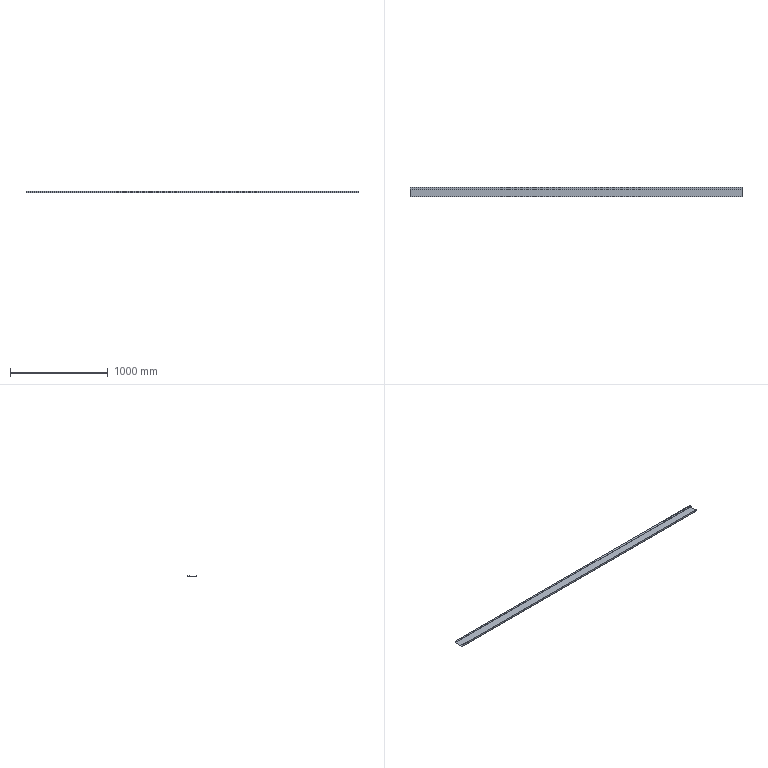Part | STEP file | Powder bin toe plate 7 | 1 solid | 18 faces | box 3390 x 100 x 20 mm | volume 779259 mm3 | plane 12 | cylinder 6 | commonest cylinder face diameters 2 x3 5 x3
STEP:
#1=CARTESIAN_POINT('',(0.,0.,0.));
#2=DIRECTION('',(0.,0.,1.));
#3=DIRECTION('',(1.,0.,0.));
#4=AXIS2_PLACEMENT_3D('',#1,#2,#3);
#5=CARTESIAN_POINT('',(-1695.,1.5,2.5));
#6=VERTEX_POINT('',#5);
#7=CARTESIAN_POINT('',(-1695.,1.5,20.));
#8=VERTEX_POINT('',#7);
#9=CARTESIAN_POINT('',(-1695.,1.5,2.5));
#10=DIRECTION('',(0.,0.,1.));
#11=VECTOR('',#10,1.);
#12=LINE('',#9,#11);
#13=CARTESIAN_POINT('',(1695.,1.5,2.5));
#14=DIRECTION('',(0.,-1.,0.));
#15=DIRECTION('',(0.,0.,-1.));
#16=AXIS2_PLACEMENT_3D('',#13,#14,#15);
#17=PLANE('',#16);
#18=CARTESIAN_POINT('',(0.,-3390.));
#19=DIRECTION('',(-1.,0.));
#20=VECTOR('',#19,1.);
#21=LINE('',#18,#20);
#22=(GEOMETRIC_REPRESENTATION_CONTEXT(2)PARAMETRIC_REPRESENTATION_CONTEXT()REPRESENTATION_CONTEXT('',''));
#23=DEFINITIONAL_REPRESENTATION('',(#21),#22);
#24=PCURVE('',#17,#23);
#25=CARTESIAN_POINT('',(-1695.,2.5,2.5));
#26=DIRECTION('',(-1.,0.,0.));
#27=DIRECTION('',(0.,0.,1.));
#28=AXIS2_PLACEMENT_3D('',#25,#26,#27);
#29=PLANE('',#28);
#30=CARTESIAN_POINT('',(0.,-1.));
#31=DIRECTION('',(1.,0.));
#32=VECTOR('',#31,1.);
#33=LINE('',#30,#32);
#34=(GEOMETRIC_REPRESENTATION_CONTEXT(2)PARAMETRIC_REPRESENTATION_CONTEXT()REPRESENTATION_CONTEXT('',''));
#35=DEFINITIONAL_REPRESENTATION('',(#33),#34);
#36=PCURVE('',#29,#35);
#37=SURFACE_CURVE('',#12,(#24,#36),.PCURVE_S1.);
#38=EDGE_CURVE('',#6,#8,#37,.T.);
#39=ORIENTED_EDGE('',*,*,#38,.T.);
#40=CARTESIAN_POINT('',(1695.,1.5,20.));
#41=VERTEX_POINT('',#40);
#42=CARTESIAN_POINT('',(1695.,1.5,20.));
#43=DIRECTION('',(-1.,0.,0.));
#44=VECTOR('',#43,1.);
#45=LINE('',#42,#44);
#46=CARTESIAN_POINT('',(-17.5,0.));
#47=DIRECTION('',(0.,-1.));
#48=VECTOR('',#47,1.);
#49=LINE('',#46,#48);
#50=(GEOMETRIC_REPRESENTATION_CONTEXT(2)PARAMETRIC_REPRESENTATION_CONTEXT()REPRESENTATION_CONTEXT('',''));
#51=DEFINITIONAL_REPRESENTATION('',(#49),#50);
#52=PCURVE('',#17,#51);
#53=CARTESIAN_POINT('',(1695.,0.,20.));
#54=DIRECTION('',(0.,0.,1.));
#55=DIRECTION('',(1.,0.,0.));
#56=AXIS2_PLACEMENT_3D('',#53,#54,#55);
#57=PLANE('',#56);
#58=CARTESIAN_POINT('',(0.,1.5));
#59=DIRECTION('',(-1.,0.));
#60=VECTOR('',#59,1.);
#61=LINE('',#58,#60);
#62=(GEOMETRIC_REPRESENTATION_CONTEXT(2)PARAMETRIC_REPRESENTATION_CONTEXT()REPRESENTATION_CONTEXT('',''));
#63=DEFINITIONAL_REPRESENTATION('',(#61),#62);
#64=PCURVE('',#57,#63);
#65=SURFACE_CURVE('',#45,(#52,#64),.PCURVE_S1.);
#66=EDGE_CURVE('',#41,#8,#65,.T.);
#67=ORIENTED_EDGE('',*,*,#66,.F.);
#68=CARTESIAN_POINT('',(1695.,1.5,2.5));
#69=VERTEX_POINT('',#68);
#70=CARTESIAN_POINT('',(1695.,1.5,2.5));
#71=DIRECTION('',(0.,0.,1.));
#72=VECTOR('',#71,1.);
#73=LINE('',#70,#72);
#74=CARTESIAN_POINT('',(0.,0.));
#75=DIRECTION('',(-1.,0.));
#76=VECTOR('',#75,1.);
#77=LINE('',#74,#76);
#78=(GEOMETRIC_REPRESENTATION_CONTEXT(2)PARAMETRIC_REPRESENTATION_CONTEXT()REPRESENTATION_CONTEXT('',''));
#79=DEFINITIONAL_REPRESENTATION('',(#77),#78);
#80=PCURVE('',#17,#79);
#81=CARTESIAN_POINT('',(1695.,2.5,2.5));
#82=DIRECTION('',(-1.,0.,0.));
#83=DIRECTION('',(0.,0.,1.));
#84=AXIS2_PLACEMENT_3D('',#81,#82,#83);
#85=PLANE('',#84);
#86=CARTESIAN_POINT('',(0.,-1.));
#87=DIRECTION('',(1.,0.));
#88=VECTOR('',#87,1.);
#89=LINE('',#86,#88);
#90=(GEOMETRIC_REPRESENTATION_CONTEXT(2)PARAMETRIC_REPRESENTATION_CONTEXT()REPRESENTATION_CONTEXT('',''));
#91=DEFINITIONAL_REPRESENTATION('',(#89),#90);
#92=PCURVE('',#85,#91);
#93=SURFACE_CURVE('',#73,(#80,#92),.PCURVE_S1.);
#94=EDGE_CURVE('',#69,#41,#93,.T.);
#95=ORIENTED_EDGE('',*,*,#94,.F.);
#96=CARTESIAN_POINT('',(1695.,1.5,2.5));
#97=DIRECTION('',(-1.,0.,0.));
#98=VECTOR('',#97,1.);
#99=LINE('',#96,#98);
#100=CARTESIAN_POINT('',(0.,0.));
#101=DIRECTION('',(0.,-1.));
#102=VECTOR('',#101,1.);
#103=LINE('',#100,#102);
#104=(GEOMETRIC_REPRESENTATION_CONTEXT(2)PARAMETRIC_REPRESENTATION_CONTEXT()REPRESENTATION_CONTEXT('',''));
#105=DEFINITIONAL_REPRESENTATION('',(#103),#104);
#106=PCURVE('',#17,#105);
#107=CARTESIAN_POINT('',(1695.,2.5,2.5));
#108=DIRECTION('',(-1.,0.,0.));
#109=DIRECTION('',(0.,0.,1.));
#110=AXIS2_PLACEMENT_3D('',#107,#108,#109);
#111=CYLINDRICAL_SURFACE('',#110,1.);
#112=CARTESIAN_POINT('',(4.712,0.));
#113=DIRECTION('',(0.,1.));
#114=VECTOR('',#113,1.);
#115=LINE('',#112,#114);
#116=(GEOMETRIC_REPRESENTATION_CONTEXT(2)PARAMETRIC_REPRESENTATION_CONTEXT()REPRESENTATION_CONTEXT('',''));
#117=DEFINITIONAL_REPRESENTATION('',(#115),#116);
#118=PCURVE('',#111,#117);
#119=SURFACE_CURVE('',#99,(#106,#118),.PCURVE_S1.);
#120=EDGE_CURVE('',#69,#6,#119,.T.);
#121=ORIENTED_EDGE('',*,*,#120,.T.);
#122=EDGE_LOOP('',(#39,#67,#95,#121));
#123=FACE_BOUND('',#122,.T.);
#124=ADVANCED_FACE('',(#123),#17,.F.);
#125=CARTESIAN_POINT('',(-1695.,0.,20.));
#126=VERTEX_POINT('',#125);
#127=CARTESIAN_POINT('',(-1695.,0.,20.));
#128=DIRECTION('',(0.,1.,0.));
#129=VECTOR('',#128,1.);
#130=LINE('',#127,#129);
#131=CARTESIAN_POINT('',(-3390.,0.));
#132=DIRECTION('',(0.,1.));
#133=VECTOR('',#132,1.);
#134=LINE('',#131,#133);
#135=(GEOMETRIC_REPRESENTATION_CONTEXT(2)PARAMETRIC_REPRESENTATION_CONTEXT()REPRESENTATION_CONTEXT('',''));
#136=DEFINITIONAL_REPRESENTATION('',(#134),#135);
#137=PCURVE('',#57,#136);
#138=CARTESIAN_POINT('',(17.5,-2.5));
#139=DIRECTION('',(0.,1.));
#140=VECTOR('',#139,1.);
#141=LINE('',#138,#140);
#142=(GEOMETRIC_REPRESENTATION_CONTEXT(2)PARAMETRIC_REPRESENTATION_CONTEXT()REPRESENTATION_CONTEXT('',''));
#143=DEFINITIONAL_REPRESENTATION('',(#141),#142);
#144=PCURVE('',#29,#143);
#145=SURFACE_CURVE('',#130,(#137,#144),.PCURVE_S1.);
#146=EDGE_CURVE('',#126,#8,#145,.T.);
#147=ORIENTED_EDGE('',*,*,#146,.F.);
#148=CARTESIAN_POINT('',(1695.,0.,20.));
#149=VERTEX_POINT('',#148);
#150=CARTESIAN_POINT('',(1695.,0.,20.));
#151=DIRECTION('',(-1.,0.,0.));
#152=VECTOR('',#151,1.);
#153=LINE('',#150,#152);
#154=CARTESIAN_POINT('',(0.,0.));
#155=DIRECTION('',(-1.,0.));
#156=VECTOR('',#155,1.);
#157=LINE('',#154,#156);
#158=(GEOMETRIC_REPRESENTATION_CONTEXT(2)PARAMETRIC_REPRESENTATION_CONTEXT()REPRESENTATION_CONTEXT('',''));
#159=DEFINITIONAL_REPRESENTATION('',(#157),#158);
#160=PCURVE('',#57,#159);
#161=CARTESIAN_POINT('',(1695.,0.,2.5));
#162=DIRECTION('',(0.,-1.,0.));
#163=DIRECTION('',(0.,0.,-1.));
#164=AXIS2_PLACEMENT_3D('',#161,#162,#163);
#165=PLANE('',#164);
#166=CARTESIAN_POINT('',(-17.5,0.));
#167=DIRECTION('',(0.,-1.));
#168=VECTOR('',#167,1.);
#169=LINE('',#166,#168);
#170=(GEOMETRIC_REPRESENTATION_CONTEXT(2)PARAMETRIC_REPRESENTATION_CONTEXT()REPRESENTATION_CONTEXT('',''));
#171=DEFINITIONAL_REPRESENTATION('',(#169),#170);
#172=PCURVE('',#165,#171);
#173=SURFACE_CURVE('',#153,(#160,#172),.PCURVE_S1.);
#174=EDGE_CURVE('',#149,#126,#173,.T.);
#175=ORIENTED_EDGE('',*,*,#174,.F.);
#176=CARTESIAN_POINT('',(1695.,0.,20.));
#177=DIRECTION('',(0.,1.,0.));
#178=VECTOR('',#177,1.);
#179=LINE('',#176,#178);
#180=CARTESIAN_POINT('',(0.,0.));
#181=DIRECTION('',(0.,1.));
#182=VECTOR('',#181,1.);
#183=LINE('',#180,#182);
#184=(GEOMETRIC_REPRESENTATION_CONTEXT(2)PARAMETRIC_REPRESENTATION_CONTEXT()REPRESENTATION_CONTEXT('',''));
#185=DEFINITIONAL_REPRESENTATION('',(#183),#184);
#186=PCURVE('',#57,#185);
#187=CARTESIAN_POINT('',(17.5,-2.5));
#188=DIRECTION('',(0.,1.));
#189=VECTOR('',#188,1.);
#190=LINE('',#187,#189);
#191=(GEOMETRIC_REPRESENTATION_CONTEXT(2)PARAMETRIC_REPRESENTATION_CONTEXT()REPRESENTATION_CONTEXT('',''));
#192=DEFINITIONAL_REPRESENTATION('',(#190),#191);
#193=PCURVE('',#85,#192);
#194=SURFACE_CURVE('',#179,(#186,#193),.PCURVE_S1.);
#195=EDGE_CURVE('',#149,#41,#194,.T.);
#196=ORIENTED_EDGE('',*,*,#195,.T.);
#197=ORIENTED_EDGE('',*,*,#66,.T.);
#198=EDGE_LOOP('',(#147,#175,#196,#197));
#199=FACE_BOUND('',#198,.T.);
#200=ADVANCED_FACE('',(#199),#57,.T.);
#201=CARTESIAN_POINT('',(-1695.,0.,2.5));
#202=VERTEX_POINT('',#201);
#203=CARTESIAN_POINT('',(-1695.,0.,2.5));
#204=DIRECTION('',(0.,0.,1.));
#205=VECTOR('',#204,1.);
#206=LINE('',#203,#205);
#207=CARTESIAN_POINT('',(0.,-3390.));
#208=DIRECTION('',(-1.,0.));
#209=VECTOR('',#208,1.);
#210=LINE('',#207,#209);
#211=(GEOMETRIC_REPRESENTATION_CONTEXT(2)PARAMETRIC_REPRESENTATION_CONTEXT()REPRESENTATION_CONTEXT('',''));
#212=DEFINITIONAL_REPRESENTATION('',(#210),#211);
#213=PCURVE('',#165,#212);
#214=CARTESIAN_POINT('',(0.,-2.5));
#215=DIRECTION('',(1.,0.));
#216=VECTOR('',#215,1.);
#217=LINE('',#214,#216);
#218=(GEOMETRIC_REPRESENTATION_CONTEXT(2)PARAMETRIC_REPRESENTATION_CONTEXT()REPRESENTATION_CONTEXT('',''));
#219=DEFINITIONAL_REPRESENTATION('',(#217),#218);
#220=PCURVE('',#29,#219);
#221=SURFACE_CURVE('',#206,(#213,#220),.PCURVE_S1.);
#222=EDGE_CURVE('',#202,#126,#221,.T.);
#223=ORIENTED_EDGE('',*,*,#222,.F.);
#224=CARTESIAN_POINT('',(1695.,0.,2.5));
#225=VERTEX_POINT('',#224);
#226=CARTESIAN_POINT('',(1695.,0.,2.5));
#227=DIRECTION('',(-1.,0.,0.));
#228=VECTOR('',#227,1.);
#229=LINE('',#226,#228);
#230=CARTESIAN_POINT('',(0.,0.));
#231=DIRECTION('',(0.,-1.));
#232=VECTOR('',#231,1.);
#233=LINE('',#230,#232);
#234=(GEOMETRIC_REPRESENTATION_CONTEXT(2)PARAMETRIC_REPRESENTATION_CONTEXT()REPRESENTATION_CONTEXT('',''));
#235=DEFINITIONAL_REPRESENTATION('',(#233),#234);
#236=PCURVE('',#165,#235);
#237=CARTESIAN_POINT('',(1695.,2.5,2.5));
#238=DIRECTION('',(-1.,0.,0.));
#239=DIRECTION('',(0.,0.,1.));
#240=AXIS2_PLACEMENT_3D('',#237,#238,#239);
#241=CYLINDRICAL_SURFACE('',#240,2.5);
#242=CARTESIAN_POINT('',(4.712,0.));
#243=DIRECTION('',(0.,1.));
#244=VECTOR('',#243,1.);
#245=LINE('',#242,#244);
#246=(GEOMETRIC_REPRESENTATION_CONTEXT(2)PARAMETRIC_REPRESENTATION_CONTEXT()REPRESENTATION_CONTEXT('',''));
#247=DEFINITIONAL_REPRESENTATION('',(#245),#246);
#248=PCURVE('',#241,#247);
#249=SURFACE_CURVE('',#229,(#236,#248),.PCURVE_S1.);
#250=EDGE_CURVE('',#225,#202,#249,.T.);
#251=ORIENTED_EDGE('',*,*,#250,.F.);
#252=CARTESIAN_POINT('',(1695.,0.,2.5));
#253=DIRECTION('',(0.,0.,1.));
#254=VECTOR('',#253,1.);
#255=LINE('',#252,#254);
#256=CARTESIAN_POINT('',(0.,0.));
#257=DIRECTION('',(-1.,0.));
#258=VECTOR('',#257,1.);
#259=LINE('',#256,#258);
#260=(GEOMETRIC_REPRESENTATION_CONTEXT(2)PARAMETRIC_REPRESENTATION_CONTEXT()REPRESENTATION_CONTEXT('',''));
#261=DEFINITIONAL_REPRESENTATION('',(#259),#260);
#262=PCURVE('',#165,#261);
#263=CARTESIAN_POINT('',(0.,-2.5));
#264=DIRECTION('',(1.,0.));
#265=VECTOR('',#264,1.);
#266=LINE('',#263,#265);
#267=(GEOMETRIC_REPRESENTATION_CONTEXT(2)PARAMETRIC_REPRESENTATION_CONTEXT()REPRESENTATION_CONTEXT('',''));
#268=DEFINITIONAL_REPRESENTATION('',(#266),#267);
#269=PCURVE('',#85,#268);
#270=SURFACE_CURVE('',#255,(#262,#269),.PCURVE_S1.);
#271=EDGE_CURVE('',#225,#149,#270,.T.);
#272=ORIENTED_EDGE('',*,*,#271,.T.);
#273=ORIENTED_EDGE('',*,*,#174,.T.);
#274=EDGE_LOOP('',(#223,#251,#272,#273));
#275=FACE_BOUND('',#274,.T.);
#276=ADVANCED_FACE('',(#275),#165,.T.);
#277=CARTESIAN_POINT('',(-1695.,2.5,0.));
#278=VERTEX_POINT('',#277);
#279=CARTESIAN_POINT('',(-1695.,2.5,2.5));
#280=DIRECTION('',(-1.,0.,0.));
#281=DIRECTION('',(0.,0.,1.));
#282=AXIS2_PLACEMENT_3D('',#279,#280,#281);
#283=CIRCLE('',#282,2.5);
#284=CARTESIAN_POINT('',(0.,3390.));
#285=DIRECTION('',(1.,0.));
#286=VECTOR('',#285,1.);
#287=LINE('',#284,#286);
#288=(GEOMETRIC_REPRESENTATION_CONTEXT(2)PARAMETRIC_REPRESENTATION_CONTEXT()REPRESENTATION_CONTEXT('',''));
#289=DEFINITIONAL_REPRESENTATION('',(#287),#288);
#290=PCURVE('',#241,#289);
#291=CARTESIAN_POINT('',(0.,0.));
#292=DIRECTION('',(1.,0.));
#293=AXIS2_PLACEMENT_2D('',#291,#292);
#294=CIRCLE('',#293,2.5);
#295=(GEOMETRIC_REPRESENTATION_CONTEXT(2)PARAMETRIC_REPRESENTATION_CONTEXT()REPRESENTATION_CONTEXT('',''));
#296=DEFINITIONAL_REPRESENTATION('',(#294),#295);
#297=PCURVE('',#29,#296);
#298=SURFACE_CURVE('',#283,(#290,#297),.PCURVE_S1.);
#299=EDGE_CURVE('',#278,#202,#298,.T.);
#300=ORIENTED_EDGE('',*,*,#299,.F.);
#301=CARTESIAN_POINT('',(1695.,2.5,0.));
#302=VERTEX_POINT('',#301);
#303=CARTESIAN_POINT('',(1695.,2.5,0.));
#304=DIRECTION('',(-1.,0.,0.));
#305=VECTOR('',#304,1.);
#306=LINE('',#303,#305);
#307=CARTESIAN_POINT('',(3.142,0.));
#308=DIRECTION('',(0.,1.));
#309=VECTOR('',#308,1.);
#310=LINE('',#307,#309);
#311=(GEOMETRIC_REPRESENTATION_CONTEXT(2)PARAMETRIC_REPRESENTATION_CONTEXT()REPRESENTATION_CONTEXT('',''));
#312=DEFINITIONAL_REPRESENTATION('',(#310),#311);
#313=PCURVE('',#241,#312);
#314=CARTESIAN_POINT('',(1695.,2.5,0.));
#315=DIRECTION('',(0.,0.,-1.));
#316=DIRECTION('',(-1.,0.,0.));
#317=AXIS2_PLACEMENT_3D('',#314,#315,#316);
#318=PLANE('',#317);
#319=CARTESIAN_POINT('',(0.,0.));
#320=DIRECTION('',(1.,0.));
#321=VECTOR('',#320,1.);
#322=LINE('',#319,#321);
#323=(GEOMETRIC_REPRESENTATION_CONTEXT(2)PARAMETRIC_REPRESENTATION_CONTEXT()REPRESENTATION_CONTEXT('',''));
#324=DEFINITIONAL_REPRESENTATION('',(#322),#323);
#325=PCURVE('',#318,#324);
#326=SURFACE_CURVE('',#306,(#313,#325),.PCURVE_S1.);
#327=EDGE_CURVE('',#302,#278,#326,.T.);
#328=ORIENTED_EDGE('',*,*,#327,.F.);
#329=CARTESIAN_POINT('',(1695.,2.5,2.5));
#330=DIRECTION('',(-1.,0.,0.));
#331=DIRECTION('',(0.,0.,1.));
#332=AXIS2_PLACEMENT_3D('',#329,#330,#331);
#333=CIRCLE('',#332,2.5);
#334=CARTESIAN_POINT('',(0.,0.));
#335=DIRECTION('',(1.,0.));
#336=VECTOR('',#335,1.);
#337=LINE('',#334,#336);
#338=(GEOMETRIC_REPRESENTATION_CONTEXT(2)PARAMETRIC_REPRESENTATION_CONTEXT()REPRESENTATION_CONTEXT('',''));
#339=DEFINITIONAL_REPRESENTATION('',(#337),#338);
#340=PCURVE('',#241,#339);
#341=CARTESIAN_POINT('',(0.,0.));
#342=DIRECTION('',(1.,0.));
#343=AXIS2_PLACEMENT_2D('',#341,#342);
#344=CIRCLE('',#343,2.5);
#345=(GEOMETRIC_REPRESENTATION_CONTEXT(2)PARAMETRIC_REPRESENTATION_CONTEXT()REPRESENTATION_CONTEXT('',''));
#346=DEFINITIONAL_REPRESENTATION('',(#344),#345);
#347=PCURVE('',#85,#346);
#348=SURFACE_CURVE('',#333,(#340,#347),.PCURVE_S1.);
#349=EDGE_CURVE('',#302,#225,#348,.T.);
#350=ORIENTED_EDGE('',*,*,#349,.T.);
#351=ORIENTED_EDGE('',*,*,#250,.T.);
#352=EDGE_LOOP('',(#300,#328,#350,#351));
#353=FACE_BOUND('',#352,.T.);
#354=ADVANCED_FACE('',(#353),#241,.T.);
#355=CARTESIAN_POINT('',(-1695.,97.5,0.));
#356=VERTEX_POINT('',#355);
#357=CARTESIAN_POINT('',(-1695.,2.5,0.));
#358=DIRECTION('',(0.,-1.,0.));
#359=VECTOR('',#358,1.);
#360=LINE('',#357,#359);
#361=CARTESIAN_POINT('',(3390.,0.));
#362=DIRECTION('',(0.,-1.));
#363=VECTOR('',#362,1.);
#364=LINE('',#361,#363);
#365=(GEOMETRIC_REPRESENTATION_CONTEXT(2)PARAMETRIC_REPRESENTATION_CONTEXT()REPRESENTATION_CONTEXT('',''));
#366=DEFINITIONAL_REPRESENTATION('',(#364),#365);
#367=PCURVE('',#318,#366);
#368=CARTESIAN_POINT('',(-2.5,0.));
#369=DIRECTION('',(0.,-1.));
#370=VECTOR('',#369,1.);
#371=LINE('',#368,#370);
#372=(GEOMETRIC_REPRESENTATION_CONTEXT(2)PARAMETRIC_REPRESENTATION_CONTEXT()REPRESENTATION_CONTEXT('',''));
#373=DEFINITIONAL_REPRESENTATION('',(#371),#372);
#374=PCURVE('',#29,#373);
#375=SURFACE_CURVE('',#360,(#367,#374),.PCURVE_S1.);
#376=EDGE_CURVE('',#356,#278,#375,.T.);
#377=ORIENTED_EDGE('',*,*,#376,.F.);
#378=CARTESIAN_POINT('',(1695.,97.5,0.));
#379=VERTEX_POINT('',#378);
#380=CARTESIAN_POINT('',(1695.,97.5,0.));
#381=DIRECTION('',(-1.,0.,0.));
#382=VECTOR('',#381,1.);
#383=LINE('',#380,#382);
#384=CARTESIAN_POINT('',(0.,95.));
#385=DIRECTION('',(1.,0.));
#386=VECTOR('',#385,1.);
#387=LINE('',#384,#386);
#388=(GEOMETRIC_REPRESENTATION_CONTEXT(2)PARAMETRIC_REPRESENTATION_CONTEXT()REPRESENTATION_CONTEXT('',''));
#389=DEFINITIONAL_REPRESENTATION('',(#387),#388);
#390=PCURVE('',#318,#389);
#391=CARTESIAN_POINT('',(1695.,97.5,2.5));
#392=DIRECTION('',(-1.,0.,0.));
#393=DIRECTION('',(0.,0.,1.));
#394=AXIS2_PLACEMENT_3D('',#391,#392,#393);
#395=CYLINDRICAL_SURFACE('',#394,2.5);
#396=CARTESIAN_POINT('',(3.142,0.));
#397=DIRECTION('',(0.,1.));
#398=VECTOR('',#397,1.);
#399=LINE('',#396,#398);
#400=(GEOMETRIC_REPRESENTATION_CONTEXT(2)PARAMETRIC_REPRESENTATION_CONTEXT()REPRESENTATION_CONTEXT('',''));
#401=DEFINITIONAL_REPRESENTATION('',(#399),#400);
#402=PCURVE('',#395,#401);
#403=SURFACE_CURVE('',#383,(#390,#402),.PCURVE_S1.);
#404=EDGE_CURVE('',#379,#356,#403,.T.);
#405=ORIENTED_EDGE('',*,*,#404,.F.);
#406=CARTESIAN_POINT('',(1695.,2.5,0.));
#407=DIRECTION('',(0.,-1.,0.));
#408=VECTOR('',#407,1.);
#409=LINE('',#406,#408);
#410=CARTESIAN_POINT('',(0.,0.));
#411=DIRECTION('',(0.,-1.));
#412=VECTOR('',#411,1.);
#413=LINE('',#410,#412);
#414=(GEOMETRIC_REPRESENTATION_CONTEXT(2)PARAMETRIC_REPRESENTATION_CONTEXT()REPRESENTATION_CONTEXT('',''));
#415=DEFINITIONAL_REPRESENTATION('',(#413),#414);
#416=PCURVE('',#318,#415);
#417=CARTESIAN_POINT('',(-2.5,0.));
#418=DIRECTION('',(0.,-1.));
#419=VECTOR('',#418,1.);
#420=LINE('',#417,#419);
#421=(GEOMETRIC_REPRESENTATION_CONTEXT(2)PARAMETRIC_REPRESENTATION_CONTEXT()REPRESENTATION_CONTEXT('',''));
#422=DEFINITIONAL_REPRESENTATION('',(#420),#421);
#423=PCURVE('',#85,#422);
#424=SURFACE_CURVE('',#409,(#416,#423),.PCURVE_S1.);
#425=EDGE_CURVE('',#379,#302,#424,.T.);
#426=ORIENTED_EDGE('',*,*,#425,.T.);
#427=ORIENTED_EDGE('',*,*,#327,.T.);
#428=EDGE_LOOP('',(#377,#405,#426,#427));
#429=FACE_BOUND('',#428,.T.);
#430=ADVANCED_FACE('',(#429),#318,.T.);
#431=CARTESIAN_POINT('',(-1695.,100.,2.5));
#432=VERTEX_POINT('',#431);
#433=CARTESIAN_POINT('',(-1695.,97.5,2.5));
#434=DIRECTION('',(-1.,0.,0.));
#435=DIRECTION('',(0.,0.,-1.));
#436=AXIS2_PLACEMENT_3D('',#433,#434,#435);
#437=CIRCLE('',#436,2.5);
#438=CARTESIAN_POINT('',(-3.142,3390.));
#439=DIRECTION('',(1.,0.));
#440=VECTOR('',#439,1.);
#441=LINE('',#438,#440);
#442=(GEOMETRIC_REPRESENTATION_CONTEXT(2)PARAMETRIC_REPRESENTATION_CONTEXT()REPRESENTATION_CONTEXT('',''));
#443=DEFINITIONAL_REPRESENTATION('',(#441),#442);
#444=PCURVE('',#395,#443);
#445=CARTESIAN_POINT('',(0.,95.));
#446=DIRECTION('',(-1.,0.));
#447=AXIS2_PLACEMENT_2D('',#445,#446);
#448=CIRCLE('',#447,2.5);
#449=(GEOMETRIC_REPRESENTATION_CONTEXT(2)PARAMETRIC_REPRESENTATION_CONTEXT()REPRESENTATION_CONTEXT('',''));
#450=DEFINITIONAL_REPRESENTATION('',(#448),#449);
#451=PCURVE('',#29,#450);
#452=SURFACE_CURVE('',#437,(#444,#451),.PCURVE_S1.);
#453=EDGE_CURVE('',#432,#356,#452,.T.);
#454=ORIENTED_EDGE('',*,*,#453,.F.);
#455=CARTESIAN_POINT('',(1695.,100.,2.5));
#456=VERTEX_POINT('',#455);
#457=CARTESIAN_POINT('',(1695.,100.,2.5));
#458=DIRECTION('',(-1.,0.,0.));
#459=VECTOR('',#458,1.);
#460=LINE('',#457,#459);
#461=CARTESIAN_POINT('',(1.571,0.));
#462=DIRECTION('',(0.,1.));
#463=VECTOR('',#462,1.);
#464=LINE('',#461,#463);
#465=(GEOMETRIC_REPRESENTATION_CONTEXT(2)PARAMETRIC_REPRESENTATION_CONTEXT()REPRESENTATION_CONTEXT('',''));
#466=DEFINITIONAL_REPRESENTATION('',(#464),#465);
#467=PCURVE('',#395,#466);
#468=CARTESIAN_POINT('',(1695.,100.,2.5));
#469=DIRECTION('',(0.,1.,0.));
#470=DIRECTION('',(0.,0.,1.));
#471=AXIS2_PLACEMENT_3D('',#468,#469,#470);
#472=PLANE('',#471);
#473=CARTESIAN_POINT('',(0.,0.));
#474=DIRECTION('',(0.,-1.));
#475=VECTOR('',#474,1.);
#476=LINE('',#473,#475);
#477=(GEOMETRIC_REPRESENTATION_CONTEXT(2)PARAMETRIC_REPRESENTATION_CONTEXT()REPRESENTATION_CONTEXT('',''));
#478=DEFINITIONAL_REPRESENTATION('',(#476),#477);
#479=PCURVE('',#472,#478);
#480=SURFACE_CURVE('',#460,(#467,#479),.PCURVE_S1.);
#481=EDGE_CURVE('',#456,#432,#480,.T.);
#482=ORIENTED_EDGE('',*,*,#481,.F.);
#483=CARTESIAN_POINT('',(1695.,97.5,2.5));
#484=DIRECTION('',(-1.,0.,0.));
#485=DIRECTION('',(0.,0.,-1.));
#486=AXIS2_PLACEMENT_3D('',#483,#484,#485);
#487=CIRCLE('',#486,2.5);
#488=CARTESIAN_POINT('',(-3.142,0.));
#489=DIRECTION('',(1.,0.));
#490=VECTOR('',#489,1.);
#491=LINE('',#488,#490);
#492=(GEOMETRIC_REPRESENTATION_CONTEXT(2)PARAMETRIC_REPRESENTATION_CONTEXT()REPRESENTATION_CONTEXT('',''));
#493=DEFINITIONAL_REPRESENTATION('',(#491),#492);
#494=PCURVE('',#395,#493);
#495=CARTESIAN_POINT('',(0.,95.));
#496=DIRECTION('',(-1.,0.));
#497=AXIS2_PLACEMENT_2D('',#495,#496);
#498=CIRCLE('',#497,2.5);
#499=(GEOMETRIC_REPRESENTATION_CONTEXT(2)PARAMETRIC_REPRESENTATION_CONTEXT()REPRESENTATION_CONTEXT('',''));
#500=DEFINITIONAL_REPRESENTATION('',(#498),#499);
#501=PCURVE('',#85,#500);
#502=SURFACE_CURVE('',#487,(#494,#501),.PCURVE_S1.);
#503=EDGE_CURVE('',#456,#379,#502,.T.);
#504=ORIENTED_EDGE('',*,*,#503,.T.);
#505=ORIENTED_EDGE('',*,*,#404,.T.);
#506=EDGE_LOOP('',(#454,#482,#504,#505));
#507=FACE_BOUND('',#506,.T.);
#508=ADVANCED_FACE('',(#507),#395,.T.);
#509=CARTESIAN_POINT('',(-1695.,100.,17.5));
#510=VERTEX_POINT('',#509);
#511=CARTESIAN_POINT('',(-1695.,100.,2.5));
#512=DIRECTION('',(0.,0.,-1.));
#513=VECTOR('',#512,1.);
#514=LINE('',#511,#513);
#515=CARTESIAN_POINT('',(0.,-3390.));
#516=DIRECTION('',(-1.,0.));
#517=VECTOR('',#516,1.);
#518=LINE('',#515,#517);
#519=(GEOMETRIC_REPRESENTATION_CONTEXT(2)PARAMETRIC_REPRESENTATION_CONTEXT()REPRESENTATION_CONTEXT('',''));
#520=DEFINITIONAL_REPRESENTATION('',(#518),#519);
#521=PCURVE('',#472,#520);
#522=CARTESIAN_POINT('',(0.,97.5));
#523=DIRECTION('',(-1.,0.));
#524=VECTOR('',#523,1.);
#525=LINE('',#522,#524);
#526=(GEOMETRIC_REPRESENTATION_CONTEXT(2)PARAMETRIC_REPRESENTATION_CONTEXT()REPRESENTATION_CONTEXT('',''));
#527=DEFINITIONAL_REPRESENTATION('',(#525),#526);
#528=PCURVE('',#29,#527);
#529=SURFACE_CURVE('',#514,(#521,#528),.PCURVE_S1.);
#530=EDGE_CURVE('',#510,#432,#529,.T.);
#531=ORIENTED_EDGE('',*,*,#530,.F.);
#532=CARTESIAN_POINT('',(1695.,100.,17.5));
#533=VERTEX_POINT('',#532);
#534=CARTESIAN_POINT('',(1695.,100.,17.5));
#535=DIRECTION('',(-1.,0.,0.));
#536=VECTOR('',#535,1.);
#537=LINE('',#534,#536);
#538=CARTESIAN_POINT('',(15.,0.));
#539=DIRECTION('',(0.,-1.));
#540=VECTOR('',#539,1.);
#541=LINE('',#538,#540);
#542=(GEOMETRIC_REPRESENTATION_CONTEXT(2)PARAMETRIC_REPRESENTATION_CONTEXT()REPRESENTATION_CONTEXT('',''));
#543=DEFINITIONAL_REPRESENTATION('',(#541),#542);
#544=PCURVE('',#472,#543);
#545=CARTESIAN_POINT('',(1695.,97.5,17.5));
#546=DIRECTION('',(-1.,0.,0.));
#547=DIRECTION('',(0.,0.,1.));
#548=AXIS2_PLACEMENT_3D('',#545,#546,#547);
#549=CYLINDRICAL_SURFACE('',#548,2.5);
#550=CARTESIAN_POINT('',(1.571,0.));
#551=DIRECTION('',(0.,1.));
#552=VECTOR('',#551,1.);
#553=LINE('',#550,#552);
#554=(GEOMETRIC_REPRESENTATION_CONTEXT(2)PARAMETRIC_REPRESENTATION_CONTEXT()REPRESENTATION_CONTEXT('',''));
#555=DEFINITIONAL_REPRESENTATION('',(#553),#554);
#556=PCURVE('',#549,#555);
#557=SURFACE_CURVE('',#537,(#544,#556),.PCURVE_S1.);
#558=EDGE_CURVE('',#533,#510,#557,.T.);
#559=ORIENTED_EDGE('',*,*,#558,.F.);
#560=CARTESIAN_POINT('',(1695.,100.,2.5));
#561=DIRECTION('',(0.,0.,-1.));
#562=VECTOR('',#561,1.);
#563=LINE('',#560,#562);
#564=CARTESIAN_POINT('',(0.,0.));
#565=DIRECTION('',(-1.,0.));
#566=VECTOR('',#565,1.);
#567=LINE('',#564,#566);
#568=(GEOMETRIC_REPRESENTATION_CONTEXT(2)PARAMETRIC_REPRESENTATION_CONTEXT()REPRESENTATION_CONTEXT('',''));
#569=DEFINITIONAL_REPRESENTATION('',(#567),#568);
#570=PCURVE('',#472,#569);
#571=CARTESIAN_POINT('',(0.,97.5));
#572=DIRECTION('',(-1.,0.));
#573=VECTOR('',#572,1.);
#574=LINE('',#571,#573);
#575=(GEOMETRIC_REPRESENTATION_CONTEXT(2)PARAMETRIC_REPRESENTATION_CONTEXT()REPRESENTATION_CONTEXT('',''));
#576=DEFINITIONAL_REPRESENTATION('',(#574),#575);
#577=PCURVE('',#85,#576);
#578=SURFACE_CURVE('',#563,(#570,#577),.PCURVE_S1.);
#579=EDGE_CURVE('',#533,#456,#578,.T.);
#580=ORIENTED_EDGE('',*,*,#579,.T.);
#581=ORIENTED_EDGE('',*,*,#481,.T.);
#582=EDGE_LOOP('',(#531,#559,#580,#581));
#583=FACE_BOUND('',#582,.T.);
#584=ADVANCED_FACE('',(#583),#472,.T.);
#585=CARTESIAN_POINT('',(-1695.,97.5,20.));
#586=VERTEX_POINT('',#585);
#587=CARTESIAN_POINT('',(-1695.,97.5,17.5));
#588=DIRECTION('',(-1.,0.,0.));
#589=DIRECTION('',(0.,0.,-1.));
#590=AXIS2_PLACEMENT_3D('',#587,#588,#589);
#591=CIRCLE('',#590,2.5);
#592=CARTESIAN_POINT('',(-3.142,3390.));
#593=DIRECTION('',(1.,0.));
#594=VECTOR('',#593,1.);
#595=LINE('',#592,#594);
#596=(GEOMETRIC_REPRESENTATION_CONTEXT(2)PARAMETRIC_REPRESENTATION_CONTEXT()REPRESENTATION_CONTEXT('',''));
#597=DEFINITIONAL_REPRESENTATION('',(#595),#596);
#598=PCURVE('',#549,#597);
#599=CARTESIAN_POINT('',(15.,95.));
#600=DIRECTION('',(-1.,0.));
#601=AXIS2_PLACEMENT_2D('',#599,#600);
#602=CIRCLE('',#601,2.5);
#603=(GEOMETRIC_REPRESENTATION_CONTEXT(2)PARAMETRIC_REPRESENTATION_CONTEXT()REPRESENTATION_CONTEXT('',''));
#604=DEFINITIONAL_REPRESENTATION('',(#602),#603);
#605=PCURVE('',#29,#604);
#606=SURFACE_CURVE('',#591,(#598,#605),.PCURVE_S1.);
#607=EDGE_CURVE('',#586,#510,#606,.T.);
#608=ORIENTED_EDGE('',*,*,#607,.F.);
#609=CARTESIAN_POINT('',(1695.,97.5,20.));
#610=VERTEX_POINT('',#609);
#611=CARTESIAN_POINT('',(1695.,97.5,20.));
#612=DIRECTION('',(-1.,0.,0.));
#613=VECTOR('',#612,1.);
#614=LINE('',#611,#613);
#615=CARTESIAN_POINT('',(0.,0.));
#616=DIRECTION('',(0.,1.));
#617=VECTOR('',#616,1.);
#618=LINE('',#615,#617);
#619=(GEOMETRIC_REPRESENTATION_CONTEXT(2)PARAMETRIC_REPRESENTATION_CONTEXT()REPRESENTATION_CONTEXT('',''));
#620=DEFINITIONAL_REPRESENTATION('',(#618),#619);
#621=PCURVE('',#549,#620);
#622=CARTESIAN_POINT('',(1695.,97.5,20.));
#623=DIRECTION('',(0.,0.,1.));
#624=DIRECTION('',(1.,0.,0.));
#625=AXIS2_PLACEMENT_3D('',#622,#623,#624);
#626=PLANE('',#625);
#627=CARTESIAN_POINT('',(0.,0.));
#628=DIRECTION('',(-1.,0.));
#629=VECTOR('',#628,1.);
#630=LINE('',#627,#629);
#631=(GEOMETRIC_REPRESENTATION_CONTEXT(2)PARAMETRIC_REPRESENTATION_CONTEXT()REPRESENTATION_CONTEXT('',''));
#632=DEFINITIONAL_REPRESENTATION('',(#630),#631);
#633=PCURVE('',#626,#632);
#634=SURFACE_CURVE('',#614,(#621,#633),.PCURVE_S1.);
#635=EDGE_CURVE('',#610,#586,#634,.T.);
#636=ORIENTED_EDGE('',*,*,#635,.F.);
#637=CARTESIAN_POINT('',(1695.,97.5,17.5));
#638=DIRECTION('',(-1.,0.,0.));
#639=DIRECTION('',(0.,0.,-1.));
#640=AXIS2_PLACEMENT_3D('',#637,#638,#639);
#641=CIRCLE('',#640,2.5);
#642=CARTESIAN_POINT('',(-3.142,0.));
#643=DIRECTION('',(1.,0.));
#644=VECTOR('',#643,1.);
#645=LINE('',#642,#644);
#646=(GEOMETRIC_REPRESENTATION_CONTEXT(2)PARAMETRIC_REPRESENTATION_CONTEXT()REPRESENTATION_CONTEXT('',''));
#647=DEFINITIONAL_REPRESENTATION('',(#645),#646);
#648=PCURVE('',#549,#647);
#649=CARTESIAN_POINT('',(15.,95.));
#650=DIRECTION('',(-1.,0.));
#651=AXIS2_PLACEMENT_2D('',#649,#650);
#652=CIRCLE('',#651,2.5);
#653=(GEOMETRIC_REPRESENTATION_CONTEXT(2)PARAMETRIC_REPRESENTATION_CONTEXT()REPRESENTATION_CONTEXT('',''));
#654=DEFINITIONAL_REPRESENTATION('',(#652),#653);
#655=PCURVE('',#85,#654);
#656=SURFACE_CURVE('',#641,(#648,#655),.PCURVE_S1.);
#657=EDGE_CURVE('',#610,#533,#656,.T.);
#658=ORIENTED_EDGE('',*,*,#657,.T.);
#659=ORIENTED_EDGE('',*,*,#558,.T.);
#660=EDGE_LOOP('',(#608,#636,#658,#659));
#661=FACE_BOUND('',#660,.T.);
#662=ADVANCED_FACE('',(#661),#549,.T.);
#663=CARTESIAN_POINT('',(-1695.,80.,20.));
#664=VERTEX_POINT('',#663);
#665=CARTESIAN_POINT('',(-1695.,97.5,20.));
#666=DIRECTION('',(0.,1.,0.));
#667=VECTOR('',#666,1.);
#668=LINE('',#665,#667);
#669=CARTESIAN_POINT('',(-3390.,0.));
#670=DIRECTION('',(0.,1.));
#671=VECTOR('',#670,1.);
#672=LINE('',#669,#671);
#673=(GEOMETRIC_REPRESENTATION_CONTEXT(2)PARAMETRIC_REPRESENTATION_CONTEXT()REPRESENTATION_CONTEXT('',''));
#674=DEFINITIONAL_REPRESENTATION('',(#672),#673);
#675=PCURVE('',#626,#674);
#676=CARTESIAN_POINT('',(17.5,95.));
#677=DIRECTION('',(0.,1.));
#678=VECTOR('',#677,1.);
#679=LINE('',#676,#678);
#680=(GEOMETRIC_REPRESENTATION_CONTEXT(2)PARAMETRIC_REPRESENTATION_CONTEXT()REPRESENTATION_CONTEXT('',''));
#681=DEFINITIONAL_REPRESENTATION('',(#679),#680);
#682=PCURVE('',#29,#681);
#683=SURFACE_CURVE('',#668,(#675,#682),.PCURVE_S1.);
#684=EDGE_CURVE('',#664,#586,#683,.T.);
#685=ORIENTED_EDGE('',*,*,#684,.F.);
#686=CARTESIAN_POINT('',(1695.,80.,20.));
#687=VERTEX_POINT('',#686);
#688=CARTESIAN_POINT('',(1695.,80.,20.));
#689=DIRECTION('',(-1.,0.,0.));
#690=VECTOR('',#689,1.);
#691=LINE('',#688,#690);
#692=CARTESIAN_POINT('',(0.,-17.5));
#693=DIRECTION('',(-1.,0.));
#694=VECTOR('',#693,1.);
#695=LINE('',#692,#694);
#696=(GEOMETRIC_REPRESENTATION_CONTEXT(2)PARAMETRIC_REPRESENTATION_CONTEXT()REPRESENTATION_CONTEXT('',''));
#697=DEFINITIONAL_REPRESENTATION('',(#695),#696);
#698=PCURVE('',#626,#697);
#699=CARTESIAN_POINT('',(1695.,80.,18.5));
#700=DIRECTION('',(0.,-1.,0.));
#701=DIRECTION('',(0.,0.,-1.));
#702=AXIS2_PLACEMENT_3D('',#699,#700,#701);
#703=PLANE('',#702);
#704=CARTESIAN_POINT('',(-1.5,0.));
#705=DIRECTION('',(0.,-1.));
#706=VECTOR('',#705,1.);
#707=LINE('',#704,#706);
#708=(GEOMETRIC_REPRESENTATION_CONTEXT(2)PARAMETRIC_REPRESENTATION_CONTEXT()REPRESENTATION_CONTEXT('',''));
#709=DEFINITIONAL_REPRESENTATION('',(#707),#708);
#710=PCURVE('',#703,#709);
#711=SURFACE_CURVE('',#691,(#698,#710),.PCURVE_S1.);
#712=EDGE_CURVE('',#687,#664,#711,.T.);
#713=ORIENTED_EDGE('',*,*,#712,.F.);
#714=CARTESIAN_POINT('',(1695.,97.5,20.));
#715=DIRECTION('',(0.,1.,0.));
#716=VECTOR('',#715,1.);
#717=LINE('',#714,#716);
#718=CARTESIAN_POINT('',(0.,0.));
#719=DIRECTION('',(0.,1.));
#720=VECTOR('',#719,1.);
#721=LINE('',#718,#720);
#722=(GEOMETRIC_REPRESENTATION_CONTEXT(2)PARAMETRIC_REPRESENTATION_CONTEXT()REPRESENTATION_CONTEXT('',''));
#723=DEFINITIONAL_REPRESENTATION('',(#721),#722);
#724=PCURVE('',#626,#723);
#725=CARTESIAN_POINT('',(17.5,95.));
#726=DIRECTION('',(0.,1.));
#727=VECTOR('',#726,1.);
#728=LINE('',#725,#727);
#729=(GEOMETRIC_REPRESENTATION_CONTEXT(2)PARAMETRIC_REPRESENTATION_CONTEXT()REPRESENTATION_CONTEXT('',''));
#730=DEFINITIONAL_REPRESENTATION('',(#728),#729);
#731=PCURVE('',#85,#730);
#732=SURFACE_CURVE('',#717,(#724,#731),.PCURVE_S1.);
#733=EDGE_CURVE('',#687,#610,#732,.T.);
#734=ORIENTED_EDGE('',*,*,#733,.T.);
#735=ORIENTED_EDGE('',*,*,#635,.T.);
#736=EDGE_LOOP('',(#685,#713,#734,#735));
#737=FACE_BOUND('',#736,.T.);
#738=ADVANCED_FACE('',(#737),#626,.T.);
#739=CARTESIAN_POINT('',(-1695.,80.,18.5));
#740=VERTEX_POINT('',#739);
#741=CARTESIAN_POINT('',(-1695.,80.,18.5));
#742=DIRECTION('',(0.,0.,1.));
#743=VECTOR('',#742,1.);
#744=LINE('',#741,#743);
#745=CARTESIAN_POINT('',(0.,-3390.));
#746=DIRECTION('',(-1.,0.));
#747=VECTOR('',#746,1.);
#748=LINE('',#745,#747);
#749=(GEOMETRIC_REPRESENTATION_CONTEXT(2)PARAMETRIC_REPRESENTATION_CONTEXT()REPRESENTATION_CONTEXT('',''));
#750=DEFINITIONAL_REPRESENTATION('',(#748),#749);
#751=PCURVE('',#703,#750);
#752=CARTESIAN_POINT('',(16.,77.5));
#753=DIRECTION('',(1.,0.));
#754=VECTOR('',#753,1.);
#755=LINE('',#752,#754);
#756=(GEOMETRIC_REPRESENTATION_CONTEXT(2)PARAMETRIC_REPRESENTATION_CONTEXT()REPRESENTATION_CONTEXT('',''));
#757=DEFINITIONAL_REPRESENTATION('',(#755),#756);
#758=PCURVE('',#29,#757);
#759=SURFACE_CURVE('',#744,(#751,#758),.PCURVE_S1.);
#760=EDGE_CURVE('',#740,#664,#759,.T.);
#761=ORIENTED_EDGE('',*,*,#760,.F.);
#762=CARTESIAN_POINT('',(1695.,80.,18.5));
#763=VERTEX_POINT('',#762);
#764=CARTESIAN_POINT('',(1695.,80.,18.5));
#765=DIRECTION('',(-1.,0.,0.));
#766=VECTOR('',#765,1.);
#767=LINE('',#764,#766);
#768=CARTESIAN_POINT('',(0.,0.));
#769=DIRECTION('',(0.,-1.));
#770=VECTOR('',#769,1.);
#771=LINE('',#768,#770);
#772=(GEOMETRIC_REPRESENTATION_CONTEXT(2)PARAMETRIC_REPRESENTATION_CONTEXT()REPRESENTATION_CONTEXT('',''));
#773=DEFINITIONAL_REPRESENTATION('',(#771),#772);
#774=PCURVE('',#703,#773);
#775=CARTESIAN_POINT('',(1695.,97.5,18.5));
#776=DIRECTION('',(0.,0.,1.));
#777=DIRECTION('',(1.,0.,0.));
#778=AXIS2_PLACEMENT_3D('',#775,#776,#777);
#779=PLANE('',#778);
#780=CARTESIAN_POINT('',(0.,-17.5));
#781=DIRECTION('',(-1.,0.));
#782=VECTOR('',#781,1.);
#783=LINE('',#780,#782);
#784=(GEOMETRIC_REPRESENTATION_CONTEXT(2)PARAMETRIC_REPRESENTATION_CONTEXT()REPRESENTATION_CONTEXT('',''));
#785=DEFINITIONAL_REPRESENTATION('',(#783),#784);
#786=PCURVE('',#779,#785);
#787=SURFACE_CURVE('',#767,(#774,#786),.PCURVE_S1.);
#788=EDGE_CURVE('',#763,#740,#787,.T.);
#789=ORIENTED_EDGE('',*,*,#788,.F.);
#790=CARTESIAN_POINT('',(1695.,80.,18.5));
#791=DIRECTION('',(0.,0.,1.));
#792=VECTOR('',#791,1.);
#793=LINE('',#790,#792);
#794=CARTESIAN_POINT('',(0.,0.));
#795=DIRECTION('',(-1.,0.));
#796=VECTOR('',#795,1.);
#797=LINE('',#794,#796);
#798=(GEOMETRIC_REPRESENTATION_CONTEXT(2)PARAMETRIC_REPRESENTATION_CONTEXT()REPRESENTATION_CONTEXT('',''));
#799=DEFINITIONAL_REPRESENTATION('',(#797),#798);
#800=PCURVE('',#703,#799);
#801=CARTESIAN_POINT('',(16.,77.5));
#802=DIRECTION('',(1.,0.));
#803=VECTOR('',#802,1.);
#804=LINE('',#801,#803);
#805=(GEOMETRIC_REPRESENTATION_CONTEXT(2)PARAMETRIC_REPRESENTATION_CONTEXT()REPRESENTATION_CONTEXT('',''));
#806=DEFINITIONAL_REPRESENTATION('',(#804),#805);
#807=PCURVE('',#85,#806);
#808=SURFACE_CURVE('',#793,(#800,#807),.PCURVE_S1.);
#809=EDGE_CURVE('',#763,#687,#808,.T.);
#810=ORIENTED_EDGE('',*,*,#809,.T.);
#811=ORIENTED_EDGE('',*,*,#712,.T.);
#812=EDGE_LOOP('',(#761,#789,#810,#811));
#813=FACE_BOUND('',#812,.T.);
#814=ADVANCED_FACE('',(#813),#703,.T.);
#815=CARTESIAN_POINT('',(-1695.,97.5,18.5));
#816=VERTEX_POINT('',#815);
#817=CARTESIAN_POINT('',(-1695.,97.5,18.5));
#818=DIRECTION('',(0.,1.,0.));
#819=VECTOR('',#818,1.);
#820=LINE('',#817,#819);
#821=CARTESIAN_POINT('',(-3390.,0.));
#822=DIRECTION('',(0.,1.));
#823=VECTOR('',#822,1.);
#824=LINE('',#821,#823);
#825=(GEOMETRIC_REPRESENTATION_CONTEXT(2)PARAMETRIC_REPRESENTATION_CONTEXT()REPRESENTATION_CONTEXT('',''));
#826=DEFINITIONAL_REPRESENTATION('',(#824),#825);
#827=PCURVE('',#779,#826);
#828=CARTESIAN_POINT('',(16.,95.));
#829=DIRECTION('',(0.,1.));
#830=VECTOR('',#829,1.);
#831=LINE('',#828,#830);
#832=(GEOMETRIC_REPRESENTATION_CONTEXT(2)PARAMETRIC_REPRESENTATION_CONTEXT()REPRESENTATION_CONTEXT('',''));
#833=DEFINITIONAL_REPRESENTATION('',(#831),#832);
#834=PCURVE('',#29,#833);
#835=SURFACE_CURVE('',#820,(#827,#834),.PCURVE_S1.);
#836=EDGE_CURVE('',#740,#816,#835,.T.);
#837=ORIENTED_EDGE('',*,*,#836,.T.);
#838=CARTESIAN_POINT('',(1695.,97.5,18.5));
#839=VERTEX_POINT('',#838);
#840=CARTESIAN_POINT('',(1695.,97.5,18.5));
#841=DIRECTION('',(-1.,0.,0.));
#842=VECTOR('',#841,1.);
#843=LINE('',#840,#842);
#844=CARTESIAN_POINT('',(0.,0.));
#845=DIRECTION('',(-1.,0.));
#846=VECTOR('',#845,1.);
#847=LINE('',#844,#846);
#848=(GEOMETRIC_REPRESENTATION_CONTEXT(2)PARAMETRIC_REPRESENTATION_CONTEXT()REPRESENTATION_CONTEXT('',''));
#849=DEFINITIONAL_REPRESENTATION('',(#847),#848);
#850=PCURVE('',#779,#849);
#851=CARTESIAN_POINT('',(1695.,97.5,17.5));
#852=DIRECTION('',(-1.,0.,0.));
#853=DIRECTION('',(0.,0.,1.));
#854=AXIS2_PLACEMENT_3D('',#851,#852,#853);
#855=CYLINDRICAL_SURFACE('',#854,1.);
#856=CARTESIAN_POINT('',(0.,0.));
#857=DIRECTION('',(0.,1.));
#858=VECTOR('',#857,1.);
#859=LINE('',#856,#858);
#860=(GEOMETRIC_REPRESENTATION_CONTEXT(2)PARAMETRIC_REPRESENTATION_CONTEXT()REPRESENTATION_CONTEXT('',''));
#861=DEFINITIONAL_REPRESENTATION('',(#859),#860);
#862=PCURVE('',#855,#861);
#863=SURFACE_CURVE('',#843,(#850,#862),.PCURVE_S1.);
#864=EDGE_CURVE('',#839,#816,#863,.T.);
#865=ORIENTED_EDGE('',*,*,#864,.F.);
#866=CARTESIAN_POINT('',(1695.,97.5,18.5));
#867=DIRECTION('',(0.,1.,0.));
#868=VECTOR('',#867,1.);
#869=LINE('',#866,#868);
#870=CARTESIAN_POINT('',(0.,0.));
#871=DIRECTION('',(0.,1.));
#872=VECTOR('',#871,1.);
#873=LINE('',#870,#872);
#874=(GEOMETRIC_REPRESENTATION_CONTEXT(2)PARAMETRIC_REPRESENTATION_CONTEXT()REPRESENTATION_CONTEXT('',''));
#875=DEFINITIONAL_REPRESENTATION('',(#873),#874);
#876=PCURVE('',#779,#875);
#877=CARTESIAN_POINT('',(16.,95.));
#878=DIRECTION('',(0.,1.));
#879=VECTOR('',#878,1.);
#880=LINE('',#877,#879);
#881=(GEOMETRIC_REPRESENTATION_CONTEXT(2)PARAMETRIC_REPRESENTATION_CONTEXT()REPRESENTATION_CONTEXT('',''));
#882=DEFINITIONAL_REPRESENTATION('',(#880),#881);
#883=PCURVE('',#85,#882);
#884=SURFACE_CURVE('',#869,(#876,#883),.PCURVE_S1.);
#885=EDGE_CURVE('',#763,#839,#884,.T.);
#886=ORIENTED_EDGE('',*,*,#885,.F.);
#887=ORIENTED_EDGE('',*,*,#788,.T.);
#888=EDGE_LOOP('',(#837,#865,#886,#887));
#889=FACE_BOUND('',#888,.T.);
#890=ADVANCED_FACE('',(#889),#779,.F.);
#891=ORIENTED_EDGE('',*,*,#864,.F.);
#892=CARTESIAN_POINT('',(1695.,98.5,17.5));
#893=VERTEX_POINT('',#892);
#894=CARTESIAN_POINT('',(1695.,97.5,17.5));
#895=DIRECTION('',(-1.,0.,0.));
#896=DIRECTION('',(0.,0.,-1.));
#897=AXIS2_PLACEMENT_3D('',#894,#895,#896);
#898=CIRCLE('',#897,1.);
#899=CARTESIAN_POINT('',(-3.142,0.));
#900=DIRECTION('',(1.,0.));
#901=VECTOR('',#900,1.);
#902=LINE('',#899,#901);
#903=(GEOMETRIC_REPRESENTATION_CONTEXT(2)PARAMETRIC_REPRESENTATION_CONTEXT()REPRESENTATION_CONTEXT('',''));
#904=DEFINITIONAL_REPRESENTATION('',(#902),#903);
#905=PCURVE('',#855,#904);
#906=CARTESIAN_POINT('',(15.,95.));
#907=DIRECTION('',(-1.,0.));
#908=AXIS2_PLACEMENT_2D('',#906,#907);
#909=CIRCLE('',#908,1.);
#910=(GEOMETRIC_REPRESENTATION_CONTEXT(2)PARAMETRIC_REPRESENTATION_CONTEXT()REPRESENTATION_CONTEXT('',''));
#911=DEFINITIONAL_REPRESENTATION('',(#909),#910);
#912=PCURVE('',#85,#911);
#913=SURFACE_CURVE('',#898,(#905,#912),.PCURVE_S1.);
#914=EDGE_CURVE('',#839,#893,#913,.T.);
#915=ORIENTED_EDGE('',*,*,#914,.T.);
#916=CARTESIAN_POINT('',(-1695.,98.5,17.5));
#917=VERTEX_POINT('',#916);
#918=CARTESIAN_POINT('',(1695.,98.5,17.5));
#919=DIRECTION('',(-1.,0.,0.));
#920=VECTOR('',#919,1.);
#921=LINE('',#918,#920);
#922=CARTESIAN_POINT('',(1.571,0.));
#923=DIRECTION('',(0.,1.));
#924=VECTOR('',#923,1.);
#925=LINE('',#922,#924);
#926=(GEOMETRIC_REPRESENTATION_CONTEXT(2)PARAMETRIC_REPRESENTATION_CONTEXT()REPRESENTATION_CONTEXT('',''));
#927=DEFINITIONAL_REPRESENTATION('',(#925),#926);
#928=PCURVE('',#855,#927);
#929=CARTESIAN_POINT('',(1695.,98.5,2.5));
#930=DIRECTION('',(0.,1.,0.));
#931=DIRECTION('',(0.,0.,1.));
#932=AXIS2_PLACEMENT_3D('',#929,#930,#931);
#933=PLANE('',#932);
#934=CARTESIAN_POINT('',(15.,0.));
#935=DIRECTION('',(0.,-1.));
#936=VECTOR('',#935,1.);
#937=LINE('',#934,#936);
#938=(GEOMETRIC_REPRESENTATION_CONTEXT(2)PARAMETRIC_REPRESENTATION_CONTEXT()REPRESENTATION_CONTEXT('',''));
#939=DEFINITIONAL_REPRESENTATION('',(#937),#938);
#940=PCURVE('',#933,#939);
#941=SURFACE_CURVE('',#921,(#928,#940),.PCURVE_S1.);
#942=EDGE_CURVE('',#893,#917,#941,.T.);
#943=ORIENTED_EDGE('',*,*,#942,.T.);
#944=CARTESIAN_POINT('',(-1695.,97.5,17.5));
#945=DIRECTION('',(-1.,0.,0.));
#946=DIRECTION('',(0.,0.,-1.));
#947=AXIS2_PLACEMENT_3D('',#944,#945,#946);
#948=CIRCLE('',#947,1.);
#949=CARTESIAN_POINT('',(-3.142,3390.));
#950=DIRECTION('',(1.,0.));
#951=VECTOR('',#950,1.);
#952=LINE('',#949,#951);
#953=(GEOMETRIC_REPRESENTATION_CONTEXT(2)PARAMETRIC_REPRESENTATION_CONTEXT()REPRESENTATION_CONTEXT('',''));
#954=DEFINITIONAL_REPRESENTATION('',(#952),#953);
#955=PCURVE('',#855,#954);
#956=CARTESIAN_POINT('',(15.,95.));
#957=DIRECTION('',(-1.,0.));
#958=AXIS2_PLACEMENT_2D('',#956,#957);
#959=CIRCLE('',#958,1.);
#960=(GEOMETRIC_REPRESENTATION_CONTEXT(2)PARAMETRIC_REPRESENTATION_CONTEXT()REPRESENTATION_CONTEXT('',''));
#961=DEFINITIONAL_REPRESENTATION('',(#959),#960);
#962=PCURVE('',#29,#961);
#963=SURFACE_CURVE('',#948,(#955,#962),.PCURVE_S1.);
#964=EDGE_CURVE('',#816,#917,#963,.T.);
#965=ORIENTED_EDGE('',*,*,#964,.F.);
#966=EDGE_LOOP('',(#891,#915,#943,#965));
#967=FACE_BOUND('',#966,.F.);
#968=ADVANCED_FACE('',(#967),#855,.F.);
#969=CARTESIAN_POINT('',(-1695.,98.5,2.5));
#970=VERTEX_POINT('',#969);
#971=CARTESIAN_POINT('',(-1695.,98.5,2.5));
#972=DIRECTION('',(0.,0.,-1.));
#973=VECTOR('',#972,1.);
#974=LINE('',#971,#973);
#975=CARTESIAN_POINT('',(0.,-3390.));
#976=DIRECTION('',(-1.,0.));
#977=VECTOR('',#976,1.);
#978=LINE('',#975,#977);
#979=(GEOMETRIC_REPRESENTATION_CONTEXT(2)PARAMETRIC_REPRESENTATION_CONTEXT()REPRESENTATION_CONTEXT('',''));
#980=DEFINITIONAL_REPRESENTATION('',(#978),#979);
#981=PCURVE('',#933,#980);
#982=CARTESIAN_POINT('',(0.,96.));
#983=DIRECTION('',(-1.,0.));
#984=VECTOR('',#983,1.);
#985=LINE('',#982,#984);
#986=(GEOMETRIC_REPRESENTATION_CONTEXT(2)PARAMETRIC_REPRESENTATION_CONTEXT()REPRESENTATION_CONTEXT('',''));
#987=DEFINITIONAL_REPRESENTATION('',(#985),#986);
#988=PCURVE('',#29,#987);
#989=SURFACE_CURVE('',#974,(#981,#988),.PCURVE_S1.);
#990=EDGE_CURVE('',#917,#970,#989,.T.);
#991=ORIENTED_EDGE('',*,*,#990,.T.);
#992=CARTESIAN_POINT('',(1695.,98.5,2.5));
#993=VERTEX_POINT('',#992);
#994=CARTESIAN_POINT('',(1695.,98.5,2.5));
#995=DIRECTION('',(-1.,0.,0.));
#996=VECTOR('',#995,1.);
#997=LINE('',#994,#996);
#998=CARTESIAN_POINT('',(0.,0.));
#999=DIRECTION('',(0.,-1.));
#1000=VECTOR('',#999,1.);
#1001=LINE('',#998,#1000);
#1002=(GEOMETRIC_REPRESENTATION_CONTEXT(2)PARAMETRIC_REPRESENTATION_CONTEXT()REPRESENTATION_CONTEXT('',''));
#1003=DEFINITIONAL_REPRESENTATION('',(#1001),#1002);
#1004=PCURVE('',#933,#1003);
#1005=CARTESIAN_POINT('',(1695.,97.5,2.5));
#1006=DIRECTION('',(-1.,0.,0.));
#1007=DIRECTION('',(0.,0.,1.));
#1008=AXIS2_PLACEMENT_3D('',#1005,#1006,#1007);
#1009=CYLINDRICAL_SURFACE('',#1008,1.);
#1010=CARTESIAN_POINT('',(1.571,0.));
#1011=DIRECTION('',(0.,1.));
#1012=VECTOR('',#1011,1.);
#1013=LINE('',#1010,#1012);
#1014=(GEOMETRIC_REPRESENTATION_CONTEXT(2)PARAMETRIC_REPRESENTATION_CONTEXT()REPRESENTATION_CONTEXT('',''));
#1015=DEFINITIONAL_REPRESENTATION('',(#1013),#1014);
#1016=PCURVE('',#1009,#1015);
#1017=SURFACE_CURVE('',#997,(#1004,#1016),.PCURVE_S1.);
#1018=EDGE_CURVE('',#993,#970,#1017,.T.);
#1019=ORIENTED_EDGE('',*,*,#1018,.F.);
#1020=CARTESIAN_POINT('',(1695.,98.5,2.5));
#1021=DIRECTION('',(0.,0.,-1.));
#1022=VECTOR('',#1021,1.);
#1023=LINE('',#1020,#1022);
#1024=CARTESIAN_POINT('',(0.,0.));
#1025=DIRECTION('',(-1.,0.));
#1026=VECTOR('',#1025,1.);
#1027=LINE('',#1024,#1026);
#1028=(GEOMETRIC_REPRESENTATION_CONTEXT(2)PARAMETRIC_REPRESENTATION_CONTEXT()REPRESENTATION_CONTEXT('',''));
#1029=DEFINITIONAL_REPRESENTATION('',(#1027),#1028);
#1030=PCURVE('',#933,#1029);
#1031=CARTESIAN_POINT('',(0.,96.));
#1032=DIRECTION('',(-1.,0.));
#1033=VECTOR('',#1032,1.);
#1034=LINE('',#1031,#1033);
#1035=(GEOMETRIC_REPRESENTATION_CONTEXT(2)PARAMETRIC_REPRESENTATION_CONTEXT()REPRESENTATION_CONTEXT('',''));
#1036=DEFINITIONAL_REPRESENTATION('',(#1034),#1035);
#1037=PCURVE('',#85,#1036);
#1038=SURFACE_CURVE('',#1023,(#1030,#1037),.PCURVE_S1.);
#1039=EDGE_CURVE('',#893,#993,#1038,.T.);
#1040=ORIENTED_EDGE('',*,*,#1039,.F.);
#1041=ORIENTED_EDGE('',*,*,#942,.T.);
#1042=EDGE_LOOP('',(#991,#1019,#1040,#1041));
#1043=FACE_BOUND('',#1042,.T.);
#1044=ADVANCED_FACE('',(#1043),#933,.F.);
#1045=ORIENTED_EDGE('',*,*,#1018,.F.);
#1046=CARTESIAN_POINT('',(1695.,97.5,1.5));
#1047=VERTEX_POINT('',#1046);
#1048=CARTESIAN_POINT('',(1695.,97.5,2.5));
#1049=DIRECTION('',(-1.,0.,0.));
#1050=DIRECTION('',(0.,0.,-1.));
#1051=AXIS2_PLACEMENT_3D('',#1048,#1049,#1050);
#1052=CIRCLE('',#1051,1.);
#1053=CARTESIAN_POINT('',(-3.142,0.));
#1054=DIRECTION('',(1.,0.));
#1055=VECTOR('',#1054,1.);
#1056=LINE('',#1053,#1055);
#1057=(GEOMETRIC_REPRESENTATION_CONTEXT(2)PARAMETRIC_REPRESENTATION_CONTEXT()REPRESENTATION_CONTEXT('',''));
#1058=DEFINITIONAL_REPRESENTATION('',(#1056),#1057);
#1059=PCURVE('',#1009,#1058);
#1060=CARTESIAN_POINT('',(0.,95.));
#1061=DIRECTION('',(-1.,0.));
#1062=AXIS2_PLACEMENT_2D('',#1060,#1061);
#1063=CIRCLE('',#1062,1.);
#1064=(GEOMETRIC_REPRESENTATION_CONTEXT(2)PARAMETRIC_REPRESENTATION_CONTEXT()REPRESENTATION_CONTEXT('',''));
#1065=DEFINITIONAL_REPRESENTATION('',(#1063),#1064);
#1066=PCURVE('',#85,#1065);
#1067=SURFACE_CURVE('',#1052,(#1059,#1066),.PCURVE_S1.);
#1068=EDGE_CURVE('',#993,#1047,#1067,.T.);
#1069=ORIENTED_EDGE('',*,*,#1068,.T.);
#1070=CARTESIAN_POINT('',(-1695.,97.5,1.5));
#1071=VERTEX_POINT('',#1070);
#1072=CARTESIAN_POINT('',(1695.,97.5,1.5));
#1073=DIRECTION('',(-1.,0.,0.));
#1074=VECTOR('',#1073,1.);
#1075=LINE('',#1072,#1074);
#1076=CARTESIAN_POINT('',(3.142,0.));
#1077=DIRECTION('',(0.,1.));
#1078=VECTOR('',#1077,1.);
#1079=LINE('',#1076,#1078);
#1080=(GEOMETRIC_REPRESENTATION_CONTEXT(2)PARAMETRIC_REPRESENTATION_CONTEXT()REPRESENTATION_CONTEXT('',''));
#1081=DEFINITIONAL_REPRESENTATION('',(#1079),#1080);
#1082=PCURVE('',#1009,#1081);
#1083=CARTESIAN_POINT('',(1695.,2.5,1.5));
#1084=DIRECTION('',(0.,0.,-1.));
#1085=DIRECTION('',(-1.,0.,0.));
#1086=AXIS2_PLACEMENT_3D('',#1083,#1084,#1085);
#1087=PLANE('',#1086);
#1088=CARTESIAN_POINT('',(0.,95.));
#1089=DIRECTION('',(1.,0.));
#1090=VECTOR('',#1089,1.);
#1091=LINE('',#1088,#1090);
#1092=(GEOMETRIC_REPRESENTATION_CONTEXT(2)PARAMETRIC_REPRESENTATION_CONTEXT()REPRESENTATION_CONTEXT('',''));
#1093=DEFINITIONAL_REPRESENTATION('',(#1091),#1092);
#1094=PCURVE('',#1087,#1093);
#1095=SURFACE_CURVE('',#1075,(#1082,#1094),.PCURVE_S1.);
#1096=EDGE_CURVE('',#1047,#1071,#1095,.T.);
#1097=ORIENTED_EDGE('',*,*,#1096,.T.);
#1098=CARTESIAN_POINT('',(-1695.,97.5,2.5));
#1099=DIRECTION('',(-1.,0.,0.));
#1100=DIRECTION('',(0.,0.,-1.));
#1101=AXIS2_PLACEMENT_3D('',#1098,#1099,#1100);
#1102=CIRCLE('',#1101,1.);
#1103=CARTESIAN_POINT('',(-3.142,3390.));
#1104=DIRECTION('',(1.,0.));
#1105=VECTOR('',#1104,1.);
#1106=LINE('',#1103,#1105);
#1107=(GEOMETRIC_REPRESENTATION_CONTEXT(2)PARAMETRIC_REPRESENTATION_CONTEXT()REPRESENTATION_CONTEXT('',''));
#1108=DEFINITIONAL_REPRESENTATION('',(#1106),#1107);
#1109=PCURVE('',#1009,#1108);
#1110=CARTESIAN_POINT('',(0.,95.));
#1111=DIRECTION('',(-1.,0.));
#1112=AXIS2_PLACEMENT_2D('',#1110,#1111);
#1113=CIRCLE('',#1112,1.);
#1114=(GEOMETRIC_REPRESENTATION_CONTEXT(2)PARAMETRIC_REPRESENTATION_CONTEXT()REPRESENTATION_CONTEXT('',''));
#1115=DEFINITIONAL_REPRESENTATION('',(#1113),#1114);
#1116=PCURVE('',#29,#1115);
#1117=SURFACE_CURVE('',#1102,(#1109,#1116),.PCURVE_S1.);
#1118=EDGE_CURVE('',#970,#1071,#1117,.T.);
#1119=ORIENTED_EDGE('',*,*,#1118,.F.);
#1120=EDGE_LOOP('',(#1045,#1069,#1097,#1119));
#1121=FACE_BOUND('',#1120,.F.);
#1122=ADVANCED_FACE('',(#1121),#1009,.F.);
#1123=CARTESIAN_POINT('',(-1695.,2.5,1.5));
#1124=VERTEX_POINT('',#1123);
#1125=CARTESIAN_POINT('',(-1695.,2.5,1.5));
#1126=DIRECTION('',(0.,-1.,0.));
#1127=VECTOR('',#1126,1.);
#1128=LINE('',#1125,#1127);
#1129=CARTESIAN_POINT('',(3390.,0.));
#1130=DIRECTION('',(0.,-1.));
#1131=VECTOR('',#1130,1.);
#1132=LINE('',#1129,#1131);
#1133=(GEOMETRIC_REPRESENTATION_CONTEXT(2)PARAMETRIC_REPRESENTATION_CONTEXT()REPRESENTATION_CONTEXT('',''));
#1134=DEFINITIONAL_REPRESENTATION('',(#1132),#1133);
#1135=PCURVE('',#1087,#1134);
#1136=CARTESIAN_POINT('',(-1.,0.));
#1137=DIRECTION('',(0.,-1.));
#1138=VECTOR('',#1137,1.);
#1139=LINE('',#1136,#1138);
#1140=(GEOMETRIC_REPRESENTATION_CONTEXT(2)PARAMETRIC_REPRESENTATION_CONTEXT()REPRESENTATION_CONTEXT('',''));
#1141=DEFINITIONAL_REPRESENTATION('',(#1139),#1140);
#1142=PCURVE('',#29,#1141);
#1143=SURFACE_CURVE('',#1128,(#1135,#1142),.PCURVE_S1.);
#1144=EDGE_CURVE('',#1071,#1124,#1143,.T.);
#1145=ORIENTED_EDGE('',*,*,#1144,.T.);
#1146=CARTESIAN_POINT('',(1695.,2.5,1.5));
#1147=VERTEX_POINT('',#1146);
#1148=CARTESIAN_POINT('',(1695.,2.5,1.5));
#1149=DIRECTION('',(-1.,0.,0.));
#1150=VECTOR('',#1149,1.);
#1151=LINE('',#1148,#1150);
#1152=CARTESIAN_POINT('',(0.,0.));
#1153=DIRECTION('',(1.,0.));
#1154=VECTOR('',#1153,1.);
#1155=LINE('',#1152,#1154);
#1156=(GEOMETRIC_REPRESENTATION_CONTEXT(2)PARAMETRIC_REPRESENTATION_CONTEXT()REPRESENTATION_CONTEXT('',''));
#1157=DEFINITIONAL_REPRESENTATION('',(#1155),#1156);
#1158=PCURVE('',#1087,#1157);
#1159=CARTESIAN_POINT('',(3.142,0.));
#1160=DIRECTION('',(0.,1.));
#1161=VECTOR('',#1160,1.);
#1162=LINE('',#1159,#1161);
#1163=(GEOMETRIC_REPRESENTATION_CONTEXT(2)PARAMETRIC_REPRESENTATION_CONTEXT()REPRESENTATION_CONTEXT('',''));
#1164=DEFINITIONAL_REPRESENTATION('',(#1162),#1163);
#1165=PCURVE('',#111,#1164);
#1166=SURFACE_CURVE('',#1151,(#1158,#1165),.PCURVE_S1.);
#1167=EDGE_CURVE('',#1147,#1124,#1166,.T.);
#1168=ORIENTED_EDGE('',*,*,#1167,.F.);
#1169=CARTESIAN_POINT('',(1695.,2.5,1.5));
#1170=DIRECTION('',(0.,-1.,0.));
#1171=VECTOR('',#1170,1.);
#1172=LINE('',#1169,#1171);
#1173=CARTESIAN_POINT('',(0.,0.));
#1174=DIRECTION('',(0.,-1.));
#1175=VECTOR('',#1174,1.);
#1176=LINE('',#1173,#1175);
#1177=(GEOMETRIC_REPRESENTATION_CONTEXT(2)PARAMETRIC_REPRESENTATION_CONTEXT()REPRESENTATION_CONTEXT('',''));
#1178=DEFINITIONAL_REPRESENTATION('',(#1176),#1177);
#1179=PCURVE('',#1087,#1178);
#1180=CARTESIAN_POINT('',(-1.,0.));
#1181=DIRECTION('',(0.,-1.));
#1182=VECTOR('',#1181,1.);
#1183=LINE('',#1180,#1182);
#1184=(GEOMETRIC_REPRESENTATION_CONTEXT(2)PARAMETRIC_REPRESENTATION_CONTEXT()REPRESENTATION_CONTEXT('',''));
#1185=DEFINITIONAL_REPRESENTATION('',(#1183),#1184);
#1186=PCURVE('',#85,#1185);
#1187=SURFACE_CURVE('',#1172,(#1179,#1186),.PCURVE_S1.);
#1188=EDGE_CURVE('',#1047,#1147,#1187,.T.);
#1189=ORIENTED_EDGE('',*,*,#1188,.F.);
#1190=ORIENTED_EDGE('',*,*,#1096,.T.);
#1191=EDGE_LOOP('',(#1145,#1168,#1189,#1190));
#1192=FACE_BOUND('',#1191,.T.);
#1193=ADVANCED_FACE('',(#1192),#1087,.F.);
#1194=ORIENTED_EDGE('',*,*,#1167,.F.);
#1195=CARTESIAN_POINT('',(1695.,2.5,2.5));
#1196=DIRECTION('',(-1.,0.,0.));
#1197=DIRECTION('',(0.,0.,-1.));
#1198=AXIS2_PLACEMENT_3D('',#1195,#1196,#1197);
#1199=CIRCLE('',#1198,1.);
#1200=CARTESIAN_POINT('',(3.142,0.));
#1201=DIRECTION('',(1.,0.));
#1202=VECTOR('',#1201,1.);
#1203=LINE('',#1200,#1202);
#1204=(GEOMETRIC_REPRESENTATION_CONTEXT(2)PARAMETRIC_REPRESENTATION_CONTEXT()REPRESENTATION_CONTEXT('',''));
#1205=DEFINITIONAL_REPRESENTATION('',(#1203),#1204);
#1206=PCURVE('',#111,#1205);
#1207=CARTESIAN_POINT('',(0.,0.));
#1208=DIRECTION('',(-1.,0.));
#1209=AXIS2_PLACEMENT_2D('',#1207,#1208);
#1210=CIRCLE('',#1209,1.);
#1211=(GEOMETRIC_REPRESENTATION_CONTEXT(2)PARAMETRIC_REPRESENTATION_CONTEXT()REPRESENTATION_CONTEXT('',''));
#1212=DEFINITIONAL_REPRESENTATION('',(#1210),#1211);
#1213=PCURVE('',#85,#1212);
#1214=SURFACE_CURVE('',#1199,(#1206,#1213),.PCURVE_S1.);
#1215=EDGE_CURVE('',#1147,#69,#1214,.T.);
#1216=ORIENTED_EDGE('',*,*,#1215,.T.);
#1217=ORIENTED_EDGE('',*,*,#120,.T.);
#1218=CARTESIAN_POINT('',(-1695.,2.5,2.5));
#1219=DIRECTION('',(-1.,0.,0.));
#1220=DIRECTION('',(0.,0.,-1.));
#1221=AXIS2_PLACEMENT_3D('',#1218,#1219,#1220);
#1222=CIRCLE('',#1221,1.);
#1223=CARTESIAN_POINT('',(3.142,3390.));
#1224=DIRECTION('',(1.,0.));
#1225=VECTOR('',#1224,1.);
#1226=LINE('',#1223,#1225);
#1227=(GEOMETRIC_REPRESENTATION_CONTEXT(2)PARAMETRIC_REPRESENTATION_CONTEXT()REPRESENTATION_CONTEXT('',''));
#1228=DEFINITIONAL_REPRESENTATION('',(#1226),#1227);
#1229=PCURVE('',#111,#1228);
#1230=CARTESIAN_POINT('',(0.,0.));
#1231=DIRECTION('',(-1.,0.));
#1232=AXIS2_PLACEMENT_2D('',#1230,#1231);
#1233=CIRCLE('',#1232,1.);
#1234=(GEOMETRIC_REPRESENTATION_CONTEXT(2)PARAMETRIC_REPRESENTATION_CONTEXT()REPRESENTATION_CONTEXT('',''));
#1235=DEFINITIONAL_REPRESENTATION('',(#1233),#1234);
#1236=PCURVE('',#29,#1235);
#1237=SURFACE_CURVE('',#1222,(#1229,#1236),.PCURVE_S1.);
#1238=EDGE_CURVE('',#1124,#6,#1237,.T.);
#1239=ORIENTED_EDGE('',*,*,#1238,.F.);
#1240=EDGE_LOOP('',(#1194,#1216,#1217,#1239));
#1241=FACE_BOUND('',#1240,.F.);
#1242=ADVANCED_FACE('',(#1241),#111,.F.);
#1243=ORIENTED_EDGE('',*,*,#94,.T.);
#1244=ORIENTED_EDGE('',*,*,#195,.F.);
#1245=ORIENTED_EDGE('',*,*,#271,.F.);
#1246=ORIENTED_EDGE('',*,*,#349,.F.);
#1247=ORIENTED_EDGE('',*,*,#425,.F.);
#1248=ORIENTED_EDGE('',*,*,#503,.F.);
#1249=ORIENTED_EDGE('',*,*,#579,.F.);
#1250=ORIENTED_EDGE('',*,*,#657,.F.);
#1251=ORIENTED_EDGE('',*,*,#733,.F.);
#1252=ORIENTED_EDGE('',*,*,#809,.F.);
#1253=ORIENTED_EDGE('',*,*,#885,.T.);
#1254=ORIENTED_EDGE('',*,*,#914,.T.);
#1255=ORIENTED_EDGE('',*,*,#1039,.T.);
#1256=ORIENTED_EDGE('',*,*,#1068,.T.);
#1257=ORIENTED_EDGE('',*,*,#1188,.T.);
#1258=ORIENTED_EDGE('',*,*,#1215,.T.);
#1259=EDGE_LOOP('',(#1243,#1244,#1245,#1246,#1247,#1248,#1249,#1250,#1251,#1252,#1253,#1254,#1255,#1256,#1257,#1258));
#1260=FACE_BOUND('',#1259,.T.);
#1261=ADVANCED_FACE('',(#1260),#85,.F.);
#1262=ORIENTED_EDGE('',*,*,#38,.F.);
#1263=ORIENTED_EDGE('',*,*,#1238,.F.);
#1264=ORIENTED_EDGE('',*,*,#1144,.F.);
#1265=ORIENTED_EDGE('',*,*,#1118,.F.);
#1266=ORIENTED_EDGE('',*,*,#990,.F.);
#1267=ORIENTED_EDGE('',*,*,#964,.F.);
#1268=ORIENTED_EDGE('',*,*,#836,.F.);
#1269=ORIENTED_EDGE('',*,*,#760,.T.);
#1270=ORIENTED_EDGE('',*,*,#684,.T.);
#1271=ORIENTED_EDGE('',*,*,#607,.T.);
#1272=ORIENTED_EDGE('',*,*,#530,.T.);
#1273=ORIENTED_EDGE('',*,*,#453,.T.);
#1274=ORIENTED_EDGE('',*,*,#376,.T.);
#1275=ORIENTED_EDGE('',*,*,#299,.T.);
#1276=ORIENTED_EDGE('',*,*,#222,.T.);
#1277=ORIENTED_EDGE('',*,*,#146,.T.);
#1278=EDGE_LOOP('',(#1262,#1263,#1264,#1265,#1266,#1267,#1268,#1269,#1270,#1271,#1272,#1273,#1274,#1275,#1276,#1277));
#1279=FACE_BOUND('',#1278,.T.);
#1280=ADVANCED_FACE('',(#1279),#29,.T.);
#1281=CLOSED_SHELL('',(#124,#200,#276,#354,#430,#508,#584,#662,#738,#814,#890,#968,#1044,#1122,#1193,#1242,#1261,#1280));
#1282=MANIFOLD_SOLID_BREP('',#1281);
#1283=(LENGTH_UNIT()NAMED_UNIT(*)SI_UNIT(.MILLI.,.METRE.));
#1284=UNCERTAINTY_MEASURE_WITH_UNIT(LENGTH_MEASURE(0.0000001),#1283,'','');
#1285=(NAMED_UNIT(*)PLANE_ANGLE_UNIT()SI_UNIT($,.RADIAN.));
#1286=(NAMED_UNIT(*)SI_UNIT($,.STERADIAN.)SOLID_ANGLE_UNIT());
#1287=(GEOMETRIC_REPRESENTATION_CONTEXT(3)GLOBAL_UNCERTAINTY_ASSIGNED_CONTEXT((#1284))GLOBAL_UNIT_ASSIGNED_CONTEXT((#1283,#1285,#1286))REPRESENTATION_CONTEXT('',''));
#1288=ADVANCED_BREP_SHAPE_REPRESENTATION('',(#4,#1282),#1287);